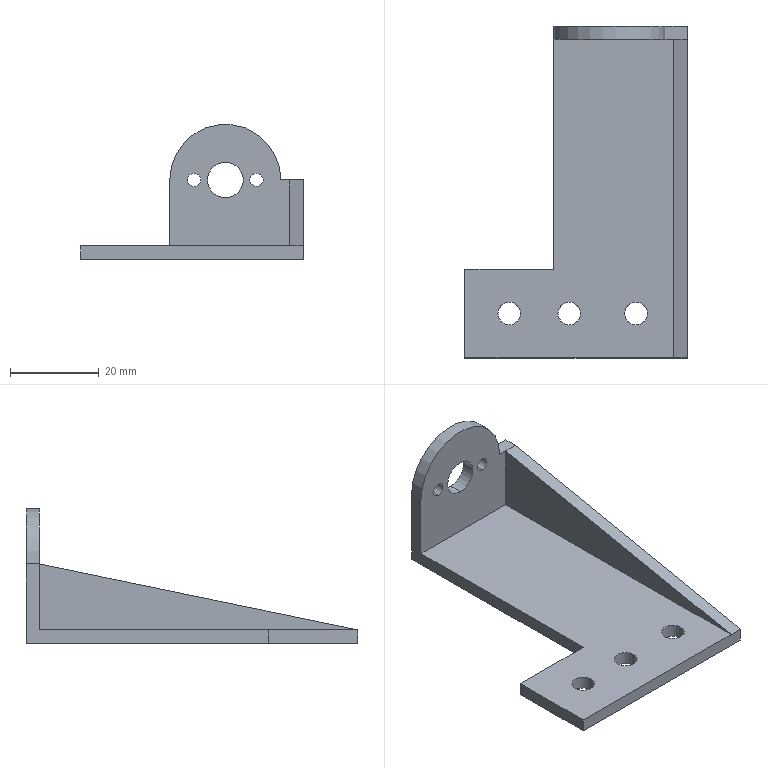Part | STEP file | Cutting motor bracket | 1 solid | 25 faces | box 50 x 74.62 x 30.335 mm | volume 11204 mm3 | cylinder 13 | plane 12 | commonest cylinder face diameters 5.1 x6 3 x4 8 x2 25 x1